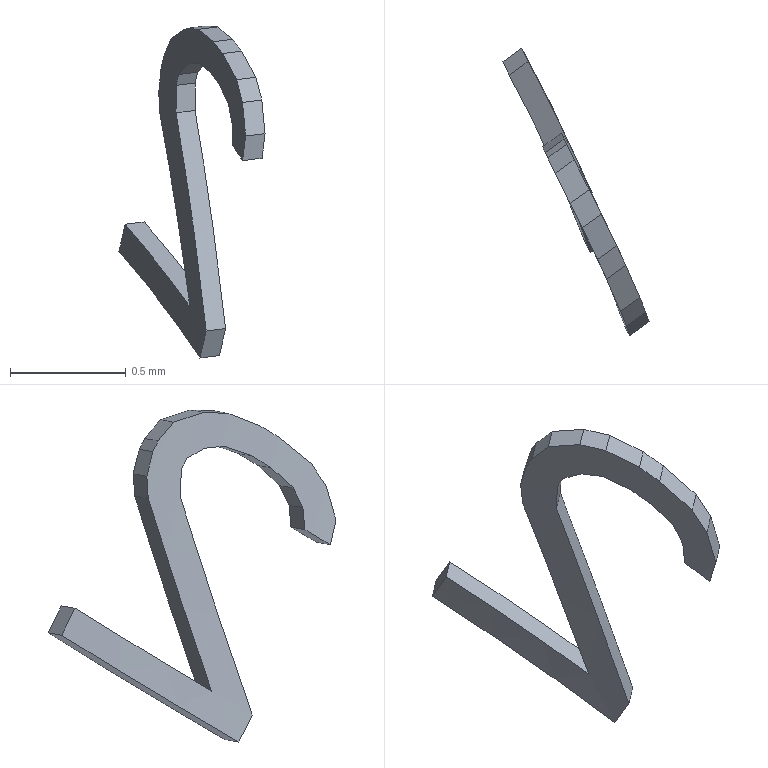Part | SolidWorks | features BaseBody 1 | 1 solid | 30 faces | box 0.631 x 1.244 x 1.435 mm | volume 0.04371 mm3 | plane 28 | cylinder 2 | commonest cylinder face diameters 16.8 x1 17 x1
STEP:
#1=CARTESIAN_POINT('',(1974.074,-240.013,991.84));
#2=VERTEX_POINT('',#1);
#3=CARTESIAN_POINT('',(1973.944,-239.701,992.783));
#4=VERTEX_POINT('',#3);
#5=CARTESIAN_POINT('',(1974.074,-240.013,991.84));
#6=CARTESIAN_POINT('',(1974.04,-239.903,992.154));
#7=CARTESIAN_POINT('',(1973.996,-239.799,992.469));
#8=CARTESIAN_POINT('',(1973.944,-239.701,992.783));
#9=B_SPLINE_CURVE_WITH_KNOTS('',3,(#5,#6,#7,#8),.UNSPECIFIED.,.F.,.F.,(4,4),(0.,1.),.UNSPECIFIED.);
#10=EDGE_CURVE('',#2,#4,#9,.T.);
#11=ORIENTED_EDGE('',*,*,#10,.T.);
#12=CARTESIAN_POINT('',(1973.944,-239.706,992.902));
#13=VERTEX_POINT('',#12);
#14=CARTESIAN_POINT('',(1973.944,-239.701,992.783));
#15=CARTESIAN_POINT('',(1973.944,-239.703,992.823));
#16=CARTESIAN_POINT('',(1973.944,-239.705,992.863));
#17=CARTESIAN_POINT('',(1973.944,-239.706,992.902));
#18=B_SPLINE_CURVE_WITH_KNOTS('',3,(#14,#15,#16,#17),.UNSPECIFIED.,.F.,.F.,(4,4),(0.,1.),.UNSPECIFIED.);
#19=EDGE_CURVE('',#4,#13,#18,.T.);
#20=ORIENTED_EDGE('',*,*,#19,.T.);
#21=CARTESIAN_POINT('',(1973.955,-239.729,992.949));
#22=VERTEX_POINT('',#21);
#23=CARTESIAN_POINT('',(1974.965,-241.915,997.345));
#24=DIRECTION('',(0.2015,-0.436,0.8771));
#25=VECTOR('',#24,1000.);
#26=LINE('',#23,#25);
#27=EDGE_CURVE('',#13,#22,#26,.T.);
#28=ORIENTED_EDGE('',*,*,#27,.T.);
#29=CARTESIAN_POINT('',(1973.992,-239.806,992.993));
#30=VERTEX_POINT('',#29);
#31=CARTESIAN_POINT('',(1973.992,-239.806,992.993));
#32=CARTESIAN_POINT('',(1973.98,-239.78,992.979));
#33=CARTESIAN_POINT('',(1973.967,-239.755,992.964));
#34=CARTESIAN_POINT('',(1973.955,-239.729,992.949));
#35=B_SPLINE_CURVE_WITH_KNOTS('',3,(#31,#32,#33,#34),.UNSPECIFIED.,.F.,.F.,(4,4),(0.,1.),.UNSPECIFIED.);
#36=EDGE_CURVE('',#30,#22,#35,.T.);
#37=ORIENTED_EDGE('',*,*,#36,.F.);
#38=CARTESIAN_POINT('',(1974.033,-239.891,993.002));
#39=VERTEX_POINT('',#38);
#40=CARTESIAN_POINT('',(1974.033,-239.891,993.002));
#41=CARTESIAN_POINT('',(1974.02,-239.863,992.999));
#42=CARTESIAN_POINT('',(1974.006,-239.834,992.996));
#43=CARTESIAN_POINT('',(1973.992,-239.806,992.993));
#44=B_SPLINE_CURVE_WITH_KNOTS('',3,(#40,#41,#42,#43),.UNSPECIFIED.,.F.,.F.,(4,4),(0.,1.),.UNSPECIFIED.);
#45=EDGE_CURVE('',#39,#30,#44,.T.);
#46=ORIENTED_EDGE('',*,*,#45,.F.);
#47=CARTESIAN_POINT('',(1974.089,-240.008,992.961));
#48=VERTEX_POINT('',#47);
#49=CARTESIAN_POINT('',(1974.089,-240.008,992.961));
#50=CARTESIAN_POINT('',(1974.071,-239.969,992.975));
#51=CARTESIAN_POINT('',(1974.052,-239.93,992.988));
#52=CARTESIAN_POINT('',(1974.033,-239.891,993.002));
#53=B_SPLINE_CURVE_WITH_KNOTS('',3,(#49,#50,#51,#52),.UNSPECIFIED.,.F.,.F.,(4,4),(0.,1.),.UNSPECIFIED.);
#54=EDGE_CURVE('',#48,#39,#53,.T.);
#55=ORIENTED_EDGE('',*,*,#54,.F.);
#56=CARTESIAN_POINT('',(1974.128,-240.093,992.91));
#57=VERTEX_POINT('',#56);
#58=CARTESIAN_POINT('',(1966.472,-243.55,992.95));
#59=DIRECTION('',(0.2015,-0.436,0.8771));
#60=DIRECTION('',(-0.7309,-0.6631,-0.1618));
#61=AXIS2_PLACEMENT_3D('',#58,#59,#60);
#62=CIRCLE('',#61,8.4);
#63=EDGE_CURVE('',#57,#48,#62,.T.);
#64=ORIENTED_EDGE('',*,*,#63,.F.);
#65=CARTESIAN_POINT('',(1974.17,-240.189,992.822));
#66=VERTEX_POINT('',#65);
#67=CARTESIAN_POINT('',(1974.17,-240.189,992.822));
#68=CARTESIAN_POINT('',(1974.156,-240.157,992.852));
#69=CARTESIAN_POINT('',(1974.142,-240.125,992.881));
#70=CARTESIAN_POINT('',(1974.128,-240.093,992.91));
#71=B_SPLINE_CURVE_WITH_KNOTS('',3,(#67,#68,#69,#70),.UNSPECIFIED.,.F.,.F.,(4,4),(0.,1.),.UNSPECIFIED.);
#72=EDGE_CURVE('',#66,#57,#71,.T.);
#73=ORIENTED_EDGE('',*,*,#72,.F.);
#74=CARTESIAN_POINT('',(1974.186,-240.231,992.737));
#75=VERTEX_POINT('',#74);
#76=CARTESIAN_POINT('',(1974.186,-240.231,992.737));
#77=CARTESIAN_POINT('',(1974.181,-240.217,992.766));
#78=CARTESIAN_POINT('',(1974.175,-240.203,992.794));
#79=CARTESIAN_POINT('',(1974.17,-240.189,992.822));
#80=B_SPLINE_CURVE_WITH_KNOTS('',3,(#76,#77,#78,#79),.UNSPECIFIED.,.F.,.F.,(4,4),(0.,1.),.UNSPECIFIED.);
#81=EDGE_CURVE('',#75,#66,#80,.T.);
#82=ORIENTED_EDGE('',*,*,#81,.F.);
#83=CARTESIAN_POINT('',(1974.188,-240.24,992.641));
#84=VERTEX_POINT('',#83);
#85=CARTESIAN_POINT('',(1974.188,-240.24,992.641));
#86=CARTESIAN_POINT('',(1974.188,-240.237,992.673));
#87=CARTESIAN_POINT('',(1974.187,-240.234,992.705));
#88=CARTESIAN_POINT('',(1974.186,-240.231,992.737));
#89=B_SPLINE_CURVE_WITH_KNOTS('',3,(#85,#86,#87,#88),.UNSPECIFIED.,.F.,.F.,(4,4),(0.,1.),.UNSPECIFIED.);
#90=EDGE_CURVE('',#84,#75,#89,.T.);
#91=ORIENTED_EDGE('',*,*,#90,.F.);
#92=CARTESIAN_POINT('',(1974.232,-240.35,992.577));
#93=VERTEX_POINT('',#92);
#94=CARTESIAN_POINT('',(1966.44,-243.481,992.81));
#95=DIRECTION('',(0.2015,-0.436,0.8771));
#96=DIRECTION('',(-0.7309,-0.6631,-0.1618));
#97=AXIS2_PLACEMENT_3D('',#94,#95,#96);
#98=CIRCLE('',#97,8.4);
#99=EDGE_CURVE('',#93,#84,#98,.T.);
#100=ORIENTED_EDGE('',*,*,#99,.F.);
#101=CARTESIAN_POINT('',(1974.244,-240.374,992.683));
#102=VERTEX_POINT('',#101);
#103=CARTESIAN_POINT('',(1974.232,-240.35,992.577));
#104=CARTESIAN_POINT('',(1974.236,-240.358,992.612));
#105=CARTESIAN_POINT('',(1974.24,-240.366,992.647));
#106=CARTESIAN_POINT('',(1974.244,-240.374,992.683));
#107=B_SPLINE_CURVE_WITH_KNOTS('',3,(#103,#104,#105,#106),.UNSPECIFIED.,.F.,.F.,(4,4),(0.,1.),.UNSPECIFIED.);
#108=EDGE_CURVE('',#93,#102,#107,.T.);
#109=ORIENTED_EDGE('',*,*,#108,.T.);
#110=CARTESIAN_POINT('',(1974.231,-240.333,992.828));
#111=VERTEX_POINT('',#110);
#112=CARTESIAN_POINT('',(1974.244,-240.374,992.683));
#113=CARTESIAN_POINT('',(1974.24,-240.36,992.731));
#114=CARTESIAN_POINT('',(1974.236,-240.347,992.78));
#115=CARTESIAN_POINT('',(1974.231,-240.333,992.828));
#116=B_SPLINE_CURVE_WITH_KNOTS('',3,(#112,#113,#114,#115),.UNSPECIFIED.,.F.,.F.,(4,4),(0.,1.),.UNSPECIFIED.);
#117=EDGE_CURVE('',#102,#111,#116,.T.);
#118=ORIENTED_EDGE('',*,*,#117,.T.);
#119=CARTESIAN_POINT('',(1974.206,-240.269,992.926));
#120=VERTEX_POINT('',#119);
#121=CARTESIAN_POINT('',(1974.231,-240.333,992.828));
#122=CARTESIAN_POINT('',(1974.223,-240.311,992.861));
#123=CARTESIAN_POINT('',(1974.214,-240.29,992.893));
#124=CARTESIAN_POINT('',(1974.206,-240.269,992.926));
#125=B_SPLINE_CURVE_WITH_KNOTS('',3,(#121,#122,#123,#124),.UNSPECIFIED.,.F.,.F.,(4,4),(0.,1.),.UNSPECIFIED.);
#126=EDGE_CURVE('',#111,#120,#125,.T.);
#127=ORIENTED_EDGE('',*,*,#126,.T.);
#128=CARTESIAN_POINT('',(1974.145,-240.13,993.039));
#129=VERTEX_POINT('',#128);
#130=CARTESIAN_POINT('',(1974.206,-240.269,992.926));
#131=CARTESIAN_POINT('',(1974.186,-240.222,992.964));
#132=CARTESIAN_POINT('',(1974.166,-240.176,993.002));
#133=CARTESIAN_POINT('',(1974.145,-240.13,993.039));
#134=B_SPLINE_CURVE_WITH_KNOTS('',3,(#130,#131,#132,#133),.UNSPECIFIED.,.F.,.F.,(4,4),(0.,1.),.UNSPECIFIED.);
#135=EDGE_CURVE('',#120,#129,#134,.T.);
#136=ORIENTED_EDGE('',*,*,#135,.T.);
#137=CARTESIAN_POINT('',(1974.106,-240.045,993.091));
#138=VERTEX_POINT('',#137);
#139=CARTESIAN_POINT('',(1966.499,-243.608,993.067));
#140=DIRECTION('',(0.2015,-0.436,0.8771));
#141=DIRECTION('',(-0.7309,-0.6631,-0.1618));
#142=AXIS2_PLACEMENT_3D('',#139,#140,#141);
#143=CIRCLE('',#142,8.4);
#144=EDGE_CURVE('',#129,#138,#143,.T.);
#145=ORIENTED_EDGE('',*,*,#144,.T.);
#146=CARTESIAN_POINT('',(1974.04,-239.908,993.144));
#147=VERTEX_POINT('',#146);
#148=CARTESIAN_POINT('',(1974.106,-240.045,993.091));
#149=CARTESIAN_POINT('',(1974.084,-239.999,993.108));
#150=CARTESIAN_POINT('',(1974.062,-239.953,993.126));
#151=CARTESIAN_POINT('',(1974.04,-239.908,993.144));
#152=B_SPLINE_CURVE_WITH_KNOTS('',3,(#148,#149,#150,#151),.UNSPECIFIED.,.F.,.F.,(4,4),(0.,1.),.UNSPECIFIED.);
#153=EDGE_CURVE('',#138,#147,#152,.T.);
#154=ORIENTED_EDGE('',*,*,#153,.T.);
#155=CARTESIAN_POINT('',(1973.987,-239.802,993.148));
#156=VERTEX_POINT('',#155);
#157=CARTESIAN_POINT('',(1974.04,-239.908,993.144));
#158=CARTESIAN_POINT('',(1974.022,-239.872,993.145));
#159=CARTESIAN_POINT('',(1974.005,-239.837,993.147));
#160=CARTESIAN_POINT('',(1973.987,-239.802,993.148));
#161=B_SPLINE_CURVE_WITH_KNOTS('',3,(#157,#158,#159,#160),.UNSPECIFIED.,.F.,.F.,(4,4),(0.,1.),.UNSPECIFIED.);
#162=EDGE_CURVE('',#147,#156,#161,.T.);
#163=ORIENTED_EDGE('',*,*,#162,.T.);
#164=CARTESIAN_POINT('',(1973.923,-239.673,993.106));
#165=VERTEX_POINT('',#164);
#166=CARTESIAN_POINT('',(1973.987,-239.802,993.148));
#167=CARTESIAN_POINT('',(1973.966,-239.759,993.134));
#168=CARTESIAN_POINT('',(1973.944,-239.716,993.12));
#169=CARTESIAN_POINT('',(1973.923,-239.673,993.106));
#170=B_SPLINE_CURVE_WITH_KNOTS('',3,(#166,#167,#168,#169),.UNSPECIFIED.,.F.,.F.,(4,4),(0.,1.),.UNSPECIFIED.);
#171=EDGE_CURVE('',#156,#165,#170,.T.);
#172=ORIENTED_EDGE('',*,*,#171,.T.);
#173=CARTESIAN_POINT('',(1973.89,-239.606,993.025));
#174=VERTEX_POINT('',#173);
#175=CARTESIAN_POINT('',(1973.923,-239.673,993.106));
#176=CARTESIAN_POINT('',(1973.912,-239.651,993.079));
#177=CARTESIAN_POINT('',(1973.901,-239.628,993.052));
#178=CARTESIAN_POINT('',(1973.89,-239.606,993.025));
#179=B_SPLINE_CURVE_WITH_KNOTS('',3,(#175,#176,#177,#178),.UNSPECIFIED.,.F.,.F.,(4,4),(0.,1.),.UNSPECIFIED.);
#180=EDGE_CURVE('',#165,#174,#179,.T.);
#181=ORIENTED_EDGE('',*,*,#180,.T.);
#182=CARTESIAN_POINT('',(1973.879,-239.583,992.978));
#183=VERTEX_POINT('',#182);
#184=CARTESIAN_POINT('',(1974.9,-241.792,997.421));
#185=DIRECTION('',(-0.2015,0.436,-0.8771));
#186=VECTOR('',#185,1000.);
#187=LINE('',#184,#186);
#188=EDGE_CURVE('',#174,#183,#187,.T.);
#189=ORIENTED_EDGE('',*,*,#188,.T.);
#190=CARTESIAN_POINT('',(1973.869,-239.557,992.872));
#191=VERTEX_POINT('',#190);
#192=CARTESIAN_POINT('',(1973.869,-239.557,992.872));
#193=CARTESIAN_POINT('',(1973.872,-239.566,992.908));
#194=CARTESIAN_POINT('',(1973.876,-239.574,992.943));
#195=CARTESIAN_POINT('',(1973.879,-239.583,992.978));
#196=B_SPLINE_CURVE_WITH_KNOTS('',3,(#192,#193,#194,#195),.UNSPECIFIED.,.F.,.F.,(4,4),(0.,1.),.UNSPECIFIED.);
#197=EDGE_CURVE('',#191,#183,#196,.T.);
#198=ORIENTED_EDGE('',*,*,#197,.F.);
#199=CARTESIAN_POINT('',(1973.875,-239.563,992.777));
#200=VERTEX_POINT('',#199);
#201=CARTESIAN_POINT('',(1973.875,-239.563,992.777));
#202=CARTESIAN_POINT('',(1973.873,-239.561,992.809));
#203=CARTESIAN_POINT('',(1973.871,-239.559,992.84));
#204=CARTESIAN_POINT('',(1973.869,-239.557,992.872));
#205=B_SPLINE_CURVE_WITH_KNOTS('',3,(#201,#202,#203,#204),.UNSPECIFIED.,.F.,.F.,(4,4),(0.,1.),.UNSPECIFIED.);
#206=EDGE_CURVE('',#200,#191,#205,.T.);
#207=ORIENTED_EDGE('',*,*,#206,.F.);
#208=CARTESIAN_POINT('',(1974.004,-239.837,991.944));
#209=VERTEX_POINT('',#208);
#210=CARTESIAN_POINT('',(1974.004,-239.837,991.944));
#211=CARTESIAN_POINT('',(1973.968,-239.741,992.221));
#212=CARTESIAN_POINT('',(1973.925,-239.65,992.499));
#213=CARTESIAN_POINT('',(1973.875,-239.563,992.777));
#214=B_SPLINE_CURVE_WITH_KNOTS('',3,(#210,#211,#212,#213),.UNSPECIFIED.,.F.,.F.,(4,4),(0.,1.),.UNSPECIFIED.);
#215=EDGE_CURVE('',#209,#200,#214,.T.);
#216=ORIENTED_EDGE('',*,*,#215,.F.);
#217=CARTESIAN_POINT('',(1973.724,-239.247,992.302));
#218=VERTEX_POINT('',#217);
#219=CARTESIAN_POINT('',(1966.274,-243.121,992.087));
#220=DIRECTION('',(0.2015,-0.436,0.8771));
#221=DIRECTION('',(-0.7309,-0.6631,-0.1618));
#222=AXIS2_PLACEMENT_3D('',#219,#220,#221);
#223=CIRCLE('',#222,8.4);
#224=EDGE_CURVE('',#209,#218,#223,.T.);
#225=ORIENTED_EDGE('',*,*,#224,.T.);
#226=CARTESIAN_POINT('',(1973.697,-239.189,992.185));
#227=VERTEX_POINT('',#226);
#228=CARTESIAN_POINT('',(1974.9,-241.792,997.421));
#229=DIRECTION('',(-0.2015,0.436,-0.8771));
#230=VECTOR('',#229,1000.);
#231=LINE('',#228,#230);
#232=EDGE_CURVE('',#218,#227,#231,.T.);
#233=ORIENTED_EDGE('',*,*,#232,.T.);
#234=CARTESIAN_POINT('',(1974.047,-239.955,991.724));
#235=VERTEX_POINT('',#234);
#236=CARTESIAN_POINT('',(1966.247,-243.063,991.97));
#237=DIRECTION('',(-0.2015,0.436,-0.8771));
#238=DIRECTION('',(-0.7309,-0.6631,-0.1618));
#239=AXIS2_PLACEMENT_3D('',#236,#237,#238);
#240=CIRCLE('',#239,8.4);
#241=EDGE_CURVE('',#227,#235,#240,.T.);
#242=ORIENTED_EDGE('',*,*,#241,.T.);
#243=CARTESIAN_POINT('',(1975.25,-242.558,996.96));
#244=DIRECTION('',(0.2015,-0.436,0.8771));
#245=VECTOR('',#244,1000.);
#246=LINE('',#243,#245);
#247=EDGE_CURVE('',#235,#2,#246,.T.);
#248=ORIENTED_EDGE('',*,*,#247,.T.);
#249=EDGE_LOOP('',(#11,#20,#28,#37,#46,#55,#64,#73,#82,#91,#100,#109,#118,#127,#136,#145,#154,#163,#172,#181,#189,#198,#207,#216,#225,#233,#242,#248));
#250=FACE_OUTER_BOUND('',#249,.T.);
#251=CARTESIAN_POINT('',(1967.45,-245.666,997.207));
#252=DIRECTION('',(0.2015,-0.436,0.8771));
#253=DIRECTION('',(-0.7309,-0.6631,-0.1618));
#254=AXIS2_PLACEMENT_3D('',#251,#252,#253);
#255=CYLINDRICAL_SURFACE('',#254,8.4);
#256=ADVANCED_FACE('',(#250),#255,.F.);
#257=CARTESIAN_POINT('',(1974.158,-239.953,991.851));
#258=VERTEX_POINT('',#257);
#259=CARTESIAN_POINT('',(1974.116,-239.983,991.846));
#260=DIRECTION('',(-0.8088,-0.5792,-0.1022));
#261=VECTOR('',#260,1000.);
#262=LINE('',#259,#261);
#263=EDGE_CURVE('',#258,#2,#262,.T.);
#264=ORIENTED_EDGE('',*,*,#263,.T.);
#265=ORIENTED_EDGE('',*,*,#247,.F.);
#266=CARTESIAN_POINT('',(1974.131,-239.895,991.734));
#267=VERTEX_POINT('',#266);
#268=CARTESIAN_POINT('',(1974.089,-239.925,991.729));
#269=DIRECTION('',(-0.8088,-0.5792,-0.1022));
#270=VECTOR('',#269,1000.);
#271=LINE('',#268,#270);
#272=EDGE_CURVE('',#267,#235,#271,.T.);
#273=ORIENTED_EDGE('',*,*,#272,.F.);
#274=CARTESIAN_POINT('',(1974.145,-239.924,991.793));
#275=DIRECTION('',(0.2015,-0.436,0.8771));
#276=VECTOR('',#275,1000.);
#277=LINE('',#274,#276);
#278=EDGE_CURVE('',#267,#258,#277,.T.);
#279=ORIENTED_EDGE('',*,*,#278,.T.);
#280=EDGE_LOOP('',(#264,#265,#273,#279));
#281=FACE_OUTER_BOUND('',#280,.T.);
#282=CARTESIAN_POINT('',(1979.641,-235.949,992.431));
#283=DIRECTION('',(0.5526,-0.6888,-0.4693));
#284=DIRECTION('',(-0.2015,0.436,-0.8771));
#285=AXIS2_PLACEMENT_3D('',#282,#283,#284);
#286=PLANE('',#285);
#287=ADVANCED_FACE('',(#281),#286,.T.);
#288=ORIENTED_EDGE('',*,*,#272,.T.);
#289=ORIENTED_EDGE('',*,*,#241,.F.);
#290=CARTESIAN_POINT('',(1973.779,-239.13,992.195));
#291=VERTEX_POINT('',#290);
#292=CARTESIAN_POINT('',(1973.738,-239.159,992.19));
#293=DIRECTION('',(-0.8088,-0.5792,-0.1022));
#294=VECTOR('',#293,1000.);
#295=LINE('',#292,#294);
#296=EDGE_CURVE('',#291,#227,#295,.T.);
#297=ORIENTED_EDGE('',*,*,#296,.F.);
#298=CARTESIAN_POINT('',(1966.247,-243.063,991.97));
#299=DIRECTION('',(-0.2015,0.436,-0.8771));
#300=DIRECTION('',(-0.7309,-0.6631,-0.1618));
#301=AXIS2_PLACEMENT_3D('',#298,#299,#300);
#302=CIRCLE('',#301,8.5);
#303=EDGE_CURVE('',#291,#267,#302,.T.);
#304=ORIENTED_EDGE('',*,*,#303,.T.);
#305=EDGE_LOOP('',(#288,#289,#297,#304));
#306=FACE_OUTER_BOUND('',#305,.T.);
#307=CARTESIAN_POINT('',(1981.656,-238.46,990.719));
#308=DIRECTION('',(-0.2015,0.436,-0.8771));
#309=DIRECTION('',(-0.5526,0.6888,0.4693));
#310=AXIS2_PLACEMENT_3D('',#307,#308,#309);
#311=PLANE('',#310);
#312=ADVANCED_FACE('',(#306),#311,.T.);
#313=ORIENTED_EDGE('',*,*,#296,.T.);
#314=ORIENTED_EDGE('',*,*,#232,.F.);
#315=CARTESIAN_POINT('',(1973.806,-239.188,992.312));
#316=VERTEX_POINT('',#315);
#317=CARTESIAN_POINT('',(1973.765,-239.217,992.307));
#318=DIRECTION('',(-0.8088,-0.5792,-0.1022));
#319=VECTOR('',#318,1000.);
#320=LINE('',#317,#319);
#321=EDGE_CURVE('',#316,#218,#320,.T.);
#322=ORIENTED_EDGE('',*,*,#321,.F.);
#323=CARTESIAN_POINT('',(1973.793,-239.159,992.254));
#324=DIRECTION('',(-0.2015,0.436,-0.8771));
#325=VECTOR('',#324,1000.);
#326=LINE('',#323,#325);
#327=EDGE_CURVE('',#316,#291,#326,.T.);
#328=ORIENTED_EDGE('',*,*,#327,.T.);
#329=EDGE_LOOP('',(#313,#314,#322,#328));
#330=FACE_OUTER_BOUND('',#329,.T.);
#331=CARTESIAN_POINT('',(1979.15,-235.361,992.987));
#332=DIRECTION('',(-0.5526,0.6888,0.4693));
#333=DIRECTION('',(0.2015,-0.436,0.8771));
#334=AXIS2_PLACEMENT_3D('',#331,#332,#333);
#335=PLANE('',#334);
#336=ADVANCED_FACE('',(#330),#335,.T.);
#337=ORIENTED_EDGE('',*,*,#321,.T.);
#338=ORIENTED_EDGE('',*,*,#224,.F.);
#339=CARTESIAN_POINT('',(1974.088,-239.777,991.955));
#340=VERTEX_POINT('',#339);
#341=CARTESIAN_POINT('',(1974.046,-239.807,991.949));
#342=DIRECTION('',(-0.8088,-0.5792,-0.1022));
#343=VECTOR('',#342,1000.);
#344=LINE('',#341,#343);
#345=EDGE_CURVE('',#340,#209,#344,.T.);
#346=ORIENTED_EDGE('',*,*,#345,.F.);
#347=CARTESIAN_POINT('',(1966.274,-243.121,992.087));
#348=DIRECTION('',(0.2015,-0.436,0.8771));
#349=DIRECTION('',(-0.7309,-0.6631,-0.1618));
#350=AXIS2_PLACEMENT_3D('',#347,#348,#349);
#351=CIRCLE('',#350,8.5);
#352=EDGE_CURVE('',#340,#316,#351,.T.);
#353=ORIENTED_EDGE('',*,*,#352,.T.);
#354=EDGE_LOOP('',(#337,#338,#346,#353));
#355=FACE_OUTER_BOUND('',#354,.T.);
#356=CARTESIAN_POINT('',(1976.862,-232.509,994.931));
#357=DIRECTION('',(0.2015,-0.436,0.8771));
#358=DIRECTION('',(0.5526,-0.6888,-0.4693));
#359=AXIS2_PLACEMENT_3D('',#356,#357,#358);
#360=PLANE('',#359);
#361=ADVANCED_FACE('',(#355),#360,.T.);
#362=ORIENTED_EDGE('',*,*,#345,.T.);
#363=ORIENTED_EDGE('',*,*,#215,.T.);
#364=CARTESIAN_POINT('',(1973.957,-239.504,992.787));
#365=VERTEX_POINT('',#364);
#366=CARTESIAN_POINT('',(1973.916,-239.534,992.782));
#367=DIRECTION('',(-0.8088,-0.5792,-0.1022));
#368=VECTOR('',#367,1000.);
#369=LINE('',#366,#368);
#370=EDGE_CURVE('',#365,#200,#369,.T.);
#371=ORIENTED_EDGE('',*,*,#370,.F.);
#372=CARTESIAN_POINT('',(1974.088,-239.777,991.955));
#373=CARTESIAN_POINT('',(1974.066,-239.72,992.121));
#374=CARTESIAN_POINT('',(1974.042,-239.664,992.287));
#375=CARTESIAN_POINT('',(1974.016,-239.609,992.454));
#376=CARTESIAN_POINT('',(1973.987,-239.556,992.621));
#377=CARTESIAN_POINT('',(1973.957,-239.504,992.787));
#378=B_SPLINE_CURVE_WITH_KNOTS('',5,(#372,#373,#374,#375,#376,#377),.UNSPECIFIED.,.F.,.F.,(6,6),(0.,1.),.UNSPECIFIED.);
#379=EDGE_CURVE('',#340,#365,#378,.T.);
#380=ORIENTED_EDGE('',*,*,#379,.F.);
#381=EDGE_LOOP('',(#362,#363,#371,#380));
#382=FACE_OUTER_BOUND('',#381,.T.);
#383=CARTESIAN_POINT('',(1979.311,-235.67,993.464));
#384=DIRECTION('',(-0.5192,0.7847,-0.3386));
#385=DIRECTION('',(-0.2763,0.2208,0.9354));
#386=AXIS2_PLACEMENT_3D('',#383,#384,#385);
#387=PLANE('',#386);
#388=ADVANCED_FACE('',(#382),#387,.T.);
#389=ORIENTED_EDGE('',*,*,#370,.T.);
#390=ORIENTED_EDGE('',*,*,#206,.T.);
#391=CARTESIAN_POINT('',(1973.951,-239.498,992.883));
#392=VERTEX_POINT('',#391);
#393=CARTESIAN_POINT('',(1973.91,-239.528,992.877));
#394=DIRECTION('',(-0.8088,-0.5792,-0.1022));
#395=VECTOR('',#394,1000.);
#396=LINE('',#393,#395);
#397=EDGE_CURVE('',#392,#191,#396,.T.);
#398=ORIENTED_EDGE('',*,*,#397,.F.);
#399=CARTESIAN_POINT('',(1973.957,-239.504,992.787));
#400=CARTESIAN_POINT('',(1973.956,-239.503,992.806));
#401=CARTESIAN_POINT('',(1973.954,-239.502,992.825));
#402=CARTESIAN_POINT('',(1973.953,-239.501,992.844));
#403=CARTESIAN_POINT('',(1973.952,-239.5,992.864));
#404=CARTESIAN_POINT('',(1973.951,-239.498,992.883));
#405=B_SPLINE_CURVE_WITH_KNOTS('',5,(#399,#400,#401,#402,#403,#404),.UNSPECIFIED.,.F.,.F.,(6,6),(0.,1.),.UNSPECIFIED.);
#406=EDGE_CURVE('',#365,#392,#405,.T.);
#407=ORIENTED_EDGE('',*,*,#406,.F.);
#408=EDGE_LOOP('',(#389,#390,#398,#407));
#409=FACE_OUTER_BOUND('',#408,.T.);
#410=CARTESIAN_POINT('',(1979.298,-235.669,993.558));
#411=DIRECTION('',(-0.5728,0.8151,-0.08642));
#412=DIRECTION('',(-0.1333,0.01137,0.991));
#413=AXIS2_PLACEMENT_3D('',#410,#411,#412);
#414=PLANE('',#413);
#415=ADVANCED_FACE('',(#409),#414,.T.);
#416=ORIENTED_EDGE('',*,*,#397,.T.);
#417=ORIENTED_EDGE('',*,*,#197,.T.);
#418=CARTESIAN_POINT('',(1973.961,-239.524,992.989));
#419=VERTEX_POINT('',#418);
#420=CARTESIAN_POINT('',(1973.92,-239.554,992.983));
#421=DIRECTION('',(-0.8088,-0.5792,-0.1022));
#422=VECTOR('',#421,1000.);
#423=LINE('',#420,#422);
#424=EDGE_CURVE('',#419,#183,#423,.T.);
#425=ORIENTED_EDGE('',*,*,#424,.F.);
#426=CARTESIAN_POINT('',(1973.951,-239.498,992.883));
#427=CARTESIAN_POINT('',(1973.953,-239.504,992.904));
#428=CARTESIAN_POINT('',(1973.955,-239.509,992.925));
#429=CARTESIAN_POINT('',(1973.957,-239.514,992.946));
#430=CARTESIAN_POINT('',(1973.959,-239.519,992.967));
#431=CARTESIAN_POINT('',(1973.961,-239.524,992.989));
#432=B_SPLINE_CURVE_WITH_KNOTS('',5,(#426,#427,#428,#429,#430,#431),.UNSPECIFIED.,.F.,.F.,(6,6),(0.,1.),.UNSPECIFIED.);
#433=EDGE_CURVE('',#392,#419,#432,.T.);
#434=ORIENTED_EDGE('',*,*,#433,.F.);
#435=EDGE_LOOP('',(#416,#417,#425,#434));
#436=FACE_OUTER_BOUND('',#435,.T.);
#437=CARTESIAN_POINT('',(1979.305,-235.697,993.664));
#438=DIRECTION('',(-0.5846,0.7727,0.2473));
#439=DIRECTION('',(0.06431,-0.2598,0.9635));
#440=AXIS2_PLACEMENT_3D('',#437,#438,#439);
#441=PLANE('',#440);
#442=ADVANCED_FACE('',(#436),#441,.T.);
#443=ORIENTED_EDGE('',*,*,#424,.T.);
#444=ORIENTED_EDGE('',*,*,#188,.F.);
#445=CARTESIAN_POINT('',(1973.972,-239.548,993.035));
#446=VERTEX_POINT('',#445);
#447=CARTESIAN_POINT('',(1973.931,-239.577,993.03));
#448=DIRECTION('',(-0.8088,-0.5792,-0.1022));
#449=VECTOR('',#448,1000.);
#450=LINE('',#447,#449);
#451=EDGE_CURVE('',#446,#174,#450,.T.);
#452=ORIENTED_EDGE('',*,*,#451,.F.);
#453=CARTESIAN_POINT('',(1973.967,-239.536,993.012));
#454=DIRECTION('',(-0.2015,0.436,-0.8771));
#455=VECTOR('',#454,1000.);
#456=LINE('',#453,#455);
#457=EDGE_CURVE('',#446,#419,#456,.T.);
#458=ORIENTED_EDGE('',*,*,#457,.T.);
#459=EDGE_LOOP('',(#443,#444,#452,#458));
#460=FACE_OUTER_BOUND('',#459,.T.);
#461=CARTESIAN_POINT('',(1979.15,-235.361,992.987));
#462=DIRECTION('',(-0.5526,0.6888,0.4693));
#463=DIRECTION('',(0.2015,-0.436,0.8771));
#464=AXIS2_PLACEMENT_3D('',#461,#462,#463);
#465=PLANE('',#464);
#466=ADVANCED_FACE('',(#460),#465,.T.);
#467=ORIENTED_EDGE('',*,*,#451,.T.);
#468=ORIENTED_EDGE('',*,*,#180,.F.);
#469=CARTESIAN_POINT('',(1974.005,-239.614,993.116));
#470=VERTEX_POINT('',#469);
#471=CARTESIAN_POINT('',(1973.964,-239.644,993.111));
#472=DIRECTION('',(-0.8088,-0.5792,-0.1022));
#473=VECTOR('',#472,1000.);
#474=LINE('',#471,#473);
#475=EDGE_CURVE('',#470,#165,#474,.T.);
#476=ORIENTED_EDGE('',*,*,#475,.F.);
#477=CARTESIAN_POINT('',(1974.005,-239.614,993.116));
#478=CARTESIAN_POINT('',(1973.998,-239.601,993.1));
#479=CARTESIAN_POINT('',(1973.992,-239.588,993.084));
#480=CARTESIAN_POINT('',(1973.985,-239.574,993.067));
#481=CARTESIAN_POINT('',(1973.979,-239.561,993.051));
#482=CARTESIAN_POINT('',(1973.972,-239.548,993.035));
#483=B_SPLINE_CURVE_WITH_KNOTS('',5,(#477,#478,#479,#480,#481,#482),.UNSPECIFIED.,.F.,.F.,(6,6),(0.,1.),.UNSPECIFIED.);
#484=EDGE_CURVE('',#470,#446,#483,.T.);
#485=ORIENTED_EDGE('',*,*,#484,.T.);
#486=EDGE_LOOP('',(#467,#468,#476,#485));
#487=FACE_OUTER_BOUND('',#486,.T.);
#488=CARTESIAN_POINT('',(1979.352,-235.785,993.791));
#489=DIRECTION('',(-0.4888,0.5653,0.6644));
#490=DIRECTION('',(0.3271,-0.5873,0.7403));
#491=AXIS2_PLACEMENT_3D('',#488,#489,#490);
#492=PLANE('',#491);
#493=ADVANCED_FACE('',(#487),#492,.T.);
#494=ORIENTED_EDGE('',*,*,#475,.T.);
#495=ORIENTED_EDGE('',*,*,#171,.F.);
#496=CARTESIAN_POINT('',(1974.069,-239.743,993.158));
#497=VERTEX_POINT('',#496);
#498=CARTESIAN_POINT('',(1974.028,-239.772,993.153));
#499=DIRECTION('',(-0.8088,-0.5792,-0.1022));
#500=VECTOR('',#499,1000.);
#501=LINE('',#498,#500);
#502=EDGE_CURVE('',#497,#156,#501,.T.);
#503=ORIENTED_EDGE('',*,*,#502,.F.);
#504=CARTESIAN_POINT('',(1974.069,-239.743,993.158));
#505=CARTESIAN_POINT('',(1974.056,-239.717,993.15));
#506=CARTESIAN_POINT('',(1974.043,-239.691,993.141));
#507=CARTESIAN_POINT('',(1974.031,-239.666,993.133));
#508=CARTESIAN_POINT('',(1974.018,-239.64,993.124));
#509=CARTESIAN_POINT('',(1974.005,-239.614,993.116));
#510=B_SPLINE_CURVE_WITH_KNOTS('',5,(#504,#505,#506,#507,#508,#509),.UNSPECIFIED.,.F.,.F.,(6,6),(0.,1.),.UNSPECIFIED.);
#511=EDGE_CURVE('',#497,#470,#510,.T.);
#512=ORIENTED_EDGE('',*,*,#511,.T.);
#513=EDGE_LOOP('',(#494,#495,#503,#512));
#514=FACE_OUTER_BOUND('',#513,.T.);
#515=CARTESIAN_POINT('',(1979.431,-235.903,993.836));
#516=DIRECTION('',(-0.2539,0.1871,0.949));
#517=DIRECTION('',(0.5305,-0.7934,0.2983));
#518=AXIS2_PLACEMENT_3D('',#515,#516,#517);
#519=PLANE('',#518);
#520=ADVANCED_FACE('',(#514),#519,.T.);
#521=ORIENTED_EDGE('',*,*,#502,.T.);
#522=ORIENTED_EDGE('',*,*,#162,.F.);
#523=CARTESIAN_POINT('',(1974.122,-239.849,993.154));
#524=VERTEX_POINT('',#523);
#525=CARTESIAN_POINT('',(1974.081,-239.878,993.149));
#526=DIRECTION('',(-0.8088,-0.5792,-0.1022));
#527=VECTOR('',#526,1000.);
#528=LINE('',#525,#527);
#529=EDGE_CURVE('',#524,#147,#528,.T.);
#530=ORIENTED_EDGE('',*,*,#529,.F.);
#531=CARTESIAN_POINT('',(1974.122,-239.849,993.154));
#532=CARTESIAN_POINT('',(1974.112,-239.827,993.155));
#533=CARTESIAN_POINT('',(1974.101,-239.806,993.156));
#534=CARTESIAN_POINT('',(1974.091,-239.785,993.157));
#535=CARTESIAN_POINT('',(1974.08,-239.764,993.158));
#536=CARTESIAN_POINT('',(1974.069,-239.743,993.158));
#537=B_SPLINE_CURVE_WITH_KNOTS('',5,(#531,#532,#533,#534,#535,#536),.UNSPECIFIED.,.F.,.F.,(6,6),(0.,1.),.UNSPECIFIED.);
#538=EDGE_CURVE('',#524,#497,#537,.T.);
#539=ORIENTED_EDGE('',*,*,#538,.T.);
#540=EDGE_LOOP('',(#521,#522,#530,#539));
#541=FACE_OUTER_BOUND('',#540,.T.);
#542=CARTESIAN_POINT('',(1979.499,-235.998,993.834));
#543=DIRECTION('',(-0.07187,-0.07511,0.9946));
#544=DIRECTION('',(0.5837,-0.8117,-0.01912));
#545=AXIS2_PLACEMENT_3D('',#542,#543,#544);
#546=PLANE('',#545);
#547=ADVANCED_FACE('',(#541),#546,.T.);
#548=ORIENTED_EDGE('',*,*,#529,.T.);
#549=ORIENTED_EDGE('',*,*,#153,.F.);
#550=CARTESIAN_POINT('',(1974.189,-239.986,993.101));
#551=VERTEX_POINT('',#550);
#552=CARTESIAN_POINT('',(1974.147,-240.016,993.096));
#553=DIRECTION('',(-0.8088,-0.5792,-0.1022));
#554=VECTOR('',#553,1000.);
#555=LINE('',#552,#554);
#556=EDGE_CURVE('',#551,#138,#555,.T.);
#557=ORIENTED_EDGE('',*,*,#556,.F.);
#558=CARTESIAN_POINT('',(1974.189,-239.986,993.101));
#559=CARTESIAN_POINT('',(1974.176,-239.958,993.112));
#560=CARTESIAN_POINT('',(1974.162,-239.931,993.122));
#561=CARTESIAN_POINT('',(1974.149,-239.903,993.133));
#562=CARTESIAN_POINT('',(1974.136,-239.876,993.144));
#563=CARTESIAN_POINT('',(1974.122,-239.849,993.154));
#564=B_SPLINE_CURVE_WITH_KNOTS('',5,(#558,#559,#560,#561,#562,#563),.UNSPECIFIED.,.F.,.F.,(6,6),(0.,1.),.UNSPECIFIED.);
#565=EDGE_CURVE('',#551,#524,#564,.T.);
#566=ORIENTED_EDGE('',*,*,#565,.T.);
#567=EDGE_LOOP('',(#548,#549,#557,#566));
#568=FACE_OUTER_BOUND('',#567,.T.);
#569=CARTESIAN_POINT('',(1979.591,-236.117,993.784));
#570=DIRECTION('',(0.1059,-0.3143,0.9434));
#571=DIRECTION('',(0.5785,-0.7522,-0.3155));
#572=AXIS2_PLACEMENT_3D('',#569,#570,#571);
#573=PLANE('',#572);
#574=ADVANCED_FACE('',(#568),#573,.T.);
#575=ORIENTED_EDGE('',*,*,#556,.T.);
#576=ORIENTED_EDGE('',*,*,#144,.F.);
#577=CARTESIAN_POINT('',(1974.228,-240.071,993.05));
#578=VERTEX_POINT('',#577);
#579=CARTESIAN_POINT('',(1974.187,-240.1,993.045));
#580=DIRECTION('',(-0.8088,-0.5792,-0.1022));
#581=VECTOR('',#580,1000.);
#582=LINE('',#579,#581);
#583=EDGE_CURVE('',#578,#129,#582,.T.);
#584=ORIENTED_EDGE('',*,*,#583,.F.);
#585=CARTESIAN_POINT('',(1966.499,-243.608,993.067));
#586=DIRECTION('',(0.2015,-0.436,0.8771));
#587=DIRECTION('',(-0.7309,-0.6631,-0.1618));
#588=AXIS2_PLACEMENT_3D('',#585,#586,#587);
#589=CIRCLE('',#588,8.5);
#590=EDGE_CURVE('',#578,#551,#589,.T.);
#591=ORIENTED_EDGE('',*,*,#590,.T.);
#592=EDGE_LOOP('',(#575,#576,#584,#591));
#593=FACE_OUTER_BOUND('',#592,.T.);
#594=CARTESIAN_POINT('',(1982.253,-239.435,991.522));
#595=DIRECTION('',(0.2015,-0.436,0.8771));
#596=DIRECTION('',(0.5526,-0.6888,-0.4693));
#597=AXIS2_PLACEMENT_3D('',#594,#595,#596);
#598=PLANE('',#597);
#599=ADVANCED_FACE('',(#593),#598,.T.);
#600=ORIENTED_EDGE('',*,*,#583,.T.);
#601=ORIENTED_EDGE('',*,*,#135,.F.);
#602=CARTESIAN_POINT('',(1974.289,-240.209,992.937));
#603=VERTEX_POINT('',#602);
#604=CARTESIAN_POINT('',(1974.247,-240.239,992.931));
#605=DIRECTION('',(-0.8088,-0.5792,-0.1022));
#606=VECTOR('',#605,1000.);
#607=LINE('',#604,#606);
#608=EDGE_CURVE('',#603,#120,#607,.T.);
#609=ORIENTED_EDGE('',*,*,#608,.F.);
#610=CARTESIAN_POINT('',(1974.289,-240.209,992.937));
#611=CARTESIAN_POINT('',(1974.277,-240.181,992.959));
#612=CARTESIAN_POINT('',(1974.265,-240.154,992.982));
#613=CARTESIAN_POINT('',(1974.253,-240.126,993.005));
#614=CARTESIAN_POINT('',(1974.241,-240.098,993.027));
#615=CARTESIAN_POINT('',(1974.228,-240.071,993.05));
#616=B_SPLINE_CURVE_WITH_KNOTS('',5,(#610,#611,#612,#613,#614,#615),.UNSPECIFIED.,.F.,.F.,(6,6),(0.,1.),.UNSPECIFIED.);
#617=EDGE_CURVE('',#603,#578,#616,.T.);
#618=ORIENTED_EDGE('',*,*,#617,.T.);
#619=EDGE_LOOP('',(#600,#601,#609,#618));
#620=FACE_OUTER_BOUND('',#619,.T.);
#621=CARTESIAN_POINT('',(1979.744,-236.303,993.626));
#622=DIRECTION('',(0.2791,-0.5309,0.8001));
#623=DIRECTION('',(0.5177,-0.6186,-0.591));
#624=AXIS2_PLACEMENT_3D('',#621,#622,#623);
#625=PLANE('',#624);
#626=ADVANCED_FACE('',(#620),#625,.T.);
#627=ORIENTED_EDGE('',*,*,#608,.T.);
#628=ORIENTED_EDGE('',*,*,#126,.F.);
#629=CARTESIAN_POINT('',(1974.315,-240.273,992.838));
#630=VERTEX_POINT('',#629);
#631=CARTESIAN_POINT('',(1974.273,-240.303,992.833));
#632=DIRECTION('',(-0.8088,-0.5792,-0.1022));
#633=VECTOR('',#632,1000.);
#634=LINE('',#631,#633);
#635=EDGE_CURVE('',#630,#111,#634,.T.);
#636=ORIENTED_EDGE('',*,*,#635,.F.);
#637=CARTESIAN_POINT('',(1974.315,-240.273,992.838));
#638=CARTESIAN_POINT('',(1974.31,-240.26,992.858));
#639=CARTESIAN_POINT('',(1974.304,-240.247,992.878));
#640=CARTESIAN_POINT('',(1974.299,-240.235,992.897));
#641=CARTESIAN_POINT('',(1974.294,-240.222,992.917));
#642=CARTESIAN_POINT('',(1974.289,-240.209,992.937));
#643=B_SPLINE_CURVE_WITH_KNOTS('',5,(#637,#638,#639,#640,#641,#642),.UNSPECIFIED.,.F.,.F.,(6,6),(0.,1.),.UNSPECIFIED.);
#644=EDGE_CURVE('',#630,#603,#643,.T.);
#645=ORIENTED_EDGE('',*,*,#644,.T.);
#646=EDGE_LOOP('',(#627,#628,#636,#645));
#647=FACE_OUTER_BOUND('',#646,.T.);
#648=CARTESIAN_POINT('',(1979.79,-236.351,993.53));
#649=DIRECTION('',(0.4307,-0.7016,0.5677));
#650=DIRECTION('',(0.4005,-0.4151,-0.8169));
#651=AXIS2_PLACEMENT_3D('',#648,#649,#650);
#652=PLANE('',#651);
#653=ADVANCED_FACE('',(#647),#652,.T.);
#654=ORIENTED_EDGE('',*,*,#635,.T.);
#655=ORIENTED_EDGE('',*,*,#117,.F.);
#656=CARTESIAN_POINT('',(1974.328,-240.314,992.693));
#657=VERTEX_POINT('',#656);
#658=CARTESIAN_POINT('',(1974.286,-240.344,992.688));
#659=DIRECTION('',(-0.8088,-0.5792,-0.1022));
#660=VECTOR('',#659,1000.);
#661=LINE('',#658,#660);
#662=EDGE_CURVE('',#657,#102,#661,.T.);
#663=ORIENTED_EDGE('',*,*,#662,.F.);
#664=CARTESIAN_POINT('',(1974.328,-240.314,992.693));
#665=CARTESIAN_POINT('',(1974.326,-240.306,992.722));
#666=CARTESIAN_POINT('',(1974.323,-240.298,992.751));
#667=CARTESIAN_POINT('',(1974.32,-240.289,992.78));
#668=CARTESIAN_POINT('',(1974.317,-240.281,992.809));
#669=CARTESIAN_POINT('',(1974.315,-240.273,992.838));
#670=B_SPLINE_CURVE_WITH_KNOTS('',5,(#664,#665,#666,#667,#668,#669),.UNSPECIFIED.,.F.,.F.,(6,6),(0.,1.),.UNSPECIFIED.);
#671=EDGE_CURVE('',#657,#630,#670,.T.);
#672=ORIENTED_EDGE('',*,*,#671,.T.);
#673=EDGE_LOOP('',(#654,#655,#663,#672));
#674=FACE_OUTER_BOUND('',#673,.T.);
#675=CARTESIAN_POINT('',(1979.827,-236.377,993.388));
#676=DIRECTION('',(0.5358,-0.7972,0.2783));
#677=DIRECTION('',(0.2426,-0.1703,-0.955));
#678=AXIS2_PLACEMENT_3D('',#675,#676,#677);
#679=PLANE('',#678);
#680=ADVANCED_FACE('',(#674),#679,.T.);
#681=ORIENTED_EDGE('',*,*,#662,.T.);
#682=ORIENTED_EDGE('',*,*,#108,.F.);
#683=CARTESIAN_POINT('',(1974.315,-240.29,992.587));
#684=VERTEX_POINT('',#683);
#685=CARTESIAN_POINT('',(1974.274,-240.32,992.582));
#686=DIRECTION('',(-0.8088,-0.5792,-0.1022));
#687=VECTOR('',#686,1000.);
#688=LINE('',#685,#687);
#689=EDGE_CURVE('',#684,#93,#688,.T.);
#690=ORIENTED_EDGE('',*,*,#689,.F.);
#691=CARTESIAN_POINT('',(1974.315,-240.29,992.587));
#692=CARTESIAN_POINT('',(1974.318,-240.295,992.608));
#693=CARTESIAN_POINT('',(1974.321,-240.3,992.63));
#694=CARTESIAN_POINT('',(1974.323,-240.305,992.651));
#695=CARTESIAN_POINT('',(1974.326,-240.31,992.672));
#696=CARTESIAN_POINT('',(1974.328,-240.314,992.693));
#697=B_SPLINE_CURVE_WITH_KNOTS('',5,(#691,#692,#693,#694,#695,#696),.UNSPECIFIED.,.F.,.F.,(6,6),(0.,1.),.UNSPECIFIED.);
#698=EDGE_CURVE('',#684,#657,#697,.T.);
#699=ORIENTED_EDGE('',*,*,#698,.T.);
#700=EDGE_LOOP('',(#681,#682,#690,#699));
#701=FACE_OUTER_BOUND('',#700,.T.);
#702=CARTESIAN_POINT('',(1979.82,-236.348,993.283));
#703=DIRECTION('',(0.5846,-0.7727,-0.2473));
#704=DIRECTION('',(-0.0643,0.2598,-0.9635));
#705=AXIS2_PLACEMENT_3D('',#702,#703,#704);
#706=PLANE('',#705);
#707=ADVANCED_FACE('',(#701),#706,.T.);
#708=CARTESIAN_POINT('',(1974.272,-240.18,992.652));
#709=VERTEX_POINT('',#708);
#710=CARTESIAN_POINT('',(1966.44,-243.481,992.81));
#711=DIRECTION('',(0.2015,-0.436,0.8771));
#712=DIRECTION('',(-0.7309,-0.6631,-0.1618));
#713=AXIS2_PLACEMENT_3D('',#710,#711,#712);
#714=CIRCLE('',#713,8.5);
#715=EDGE_CURVE('',#684,#709,#714,.T.);
#716=ORIENTED_EDGE('',*,*,#715,.F.);
#717=ORIENTED_EDGE('',*,*,#689,.T.);
#718=ORIENTED_EDGE('',*,*,#99,.T.);
#719=CARTESIAN_POINT('',(1974.23,-240.21,992.647));
#720=DIRECTION('',(-0.8088,-0.5792,-0.1022));
#721=VECTOR('',#720,1000.);
#722=LINE('',#719,#721);
#723=EDGE_CURVE('',#709,#84,#722,.T.);
#724=ORIENTED_EDGE('',*,*,#723,.F.);
#725=EDGE_LOOP('',(#716,#717,#718,#724));
#726=FACE_OUTER_BOUND('',#725,.T.);
#727=CARTESIAN_POINT('',(1976.827,-232.617,995.825));
#728=DIRECTION('',(0.2015,-0.436,0.8771));
#729=DIRECTION('',(0.5526,-0.6888,-0.4693));
#730=AXIS2_PLACEMENT_3D('',#727,#728,#729);
#731=PLANE('',#730);
#732=ADVANCED_FACE('',(#726),#731,.F.);
#733=ORIENTED_EDGE('',*,*,#723,.T.);
#734=ORIENTED_EDGE('',*,*,#90,.T.);
#735=CARTESIAN_POINT('',(1974.27,-240.171,992.748));
#736=VERTEX_POINT('',#735);
#737=CARTESIAN_POINT('',(1974.228,-240.201,992.742));
#738=DIRECTION('',(-0.8088,-0.5792,-0.1022));
#739=VECTOR('',#738,1000.);
#740=LINE('',#737,#739);
#741=EDGE_CURVE('',#736,#75,#740,.T.);
#742=ORIENTED_EDGE('',*,*,#741,.F.);
#743=CARTESIAN_POINT('',(1974.272,-240.18,992.652));
#744=CARTESIAN_POINT('',(1974.271,-240.178,992.671));
#745=CARTESIAN_POINT('',(1974.271,-240.177,992.69));
#746=CARTESIAN_POINT('',(1974.271,-240.175,992.709));
#747=CARTESIAN_POINT('',(1974.27,-240.173,992.728));
#748=CARTESIAN_POINT('',(1974.27,-240.171,992.748));
#749=B_SPLINE_CURVE_WITH_KNOTS('',5,(#743,#744,#745,#746,#747,#748),.UNSPECIFIED.,.F.,.F.,(6,6),(0.,1.),.UNSPECIFIED.);
#750=EDGE_CURVE('',#709,#736,#749,.T.);
#751=ORIENTED_EDGE('',*,*,#750,.F.);
#752=EDGE_LOOP('',(#733,#734,#742,#751));
#753=FACE_OUTER_BOUND('',#752,.T.);
#754=CARTESIAN_POINT('',(1979.735,-236.258,993.438));
#755=DIRECTION('',(-0.5728,0.8151,-0.08642));
#756=DIRECTION('',(-0.1333,0.01136,0.991));
#757=AXIS2_PLACEMENT_3D('',#754,#755,#756);
#758=PLANE('',#757);
#759=ADVANCED_FACE('',(#753),#758,.T.);
#760=ORIENTED_EDGE('',*,*,#741,.T.);
#761=ORIENTED_EDGE('',*,*,#81,.T.);
#762=CARTESIAN_POINT('',(1974.253,-240.13,992.833));
#763=VERTEX_POINT('',#762);
#764=CARTESIAN_POINT('',(1974.211,-240.16,992.828));
#765=DIRECTION('',(-0.8088,-0.5792,-0.1022));
#766=VECTOR('',#765,1000.);
#767=LINE('',#764,#766);
#768=EDGE_CURVE('',#763,#66,#767,.T.);
#769=ORIENTED_EDGE('',*,*,#768,.F.);
#770=CARTESIAN_POINT('',(1974.27,-240.171,992.748));
#771=CARTESIAN_POINT('',(1974.266,-240.163,992.765));
#772=CARTESIAN_POINT('',(1974.263,-240.155,992.782));
#773=CARTESIAN_POINT('',(1974.26,-240.146,992.799));
#774=CARTESIAN_POINT('',(1974.256,-240.138,992.816));
#775=CARTESIAN_POINT('',(1974.253,-240.13,992.833));
#776=B_SPLINE_CURVE_WITH_KNOTS('',5,(#770,#771,#772,#773,#774,#775),.UNSPECIFIED.,.F.,.F.,(6,6),(0.,1.),.UNSPECIFIED.);
#777=EDGE_CURVE('',#736,#763,#776,.T.);
#778=ORIENTED_EDGE('',*,*,#777,.F.);
#779=EDGE_LOOP('',(#760,#761,#769,#778));
#780=FACE_OUTER_BOUND('',#779,.T.);
#781=CARTESIAN_POINT('',(1979.702,-236.227,993.521));
#782=DIRECTION('',(-0.4775,0.7481,-0.4609));
#783=DIRECTION('',(-0.3434,0.3239,0.8816));
#784=AXIS2_PLACEMENT_3D('',#781,#782,#783);
#785=PLANE('',#784);
#786=ADVANCED_FACE('',(#780),#785,.T.);
#787=ORIENTED_EDGE('',*,*,#768,.T.);
#788=ORIENTED_EDGE('',*,*,#72,.T.);
#789=CARTESIAN_POINT('',(1974.211,-240.034,992.92));
#790=VERTEX_POINT('',#789);
#791=CARTESIAN_POINT('',(1974.169,-240.064,992.915));
#792=DIRECTION('',(-0.8088,-0.5792,-0.1022));
#793=VECTOR('',#792,1000.);
#794=LINE('',#791,#793);
#795=EDGE_CURVE('',#790,#57,#794,.T.);
#796=ORIENTED_EDGE('',*,*,#795,.F.);
#797=CARTESIAN_POINT('',(1974.253,-240.13,992.833));
#798=CARTESIAN_POINT('',(1974.245,-240.11,992.85));
#799=CARTESIAN_POINT('',(1974.236,-240.091,992.868));
#800=CARTESIAN_POINT('',(1974.228,-240.072,992.885));
#801=CARTESIAN_POINT('',(1974.219,-240.053,992.903));
#802=CARTESIAN_POINT('',(1974.211,-240.034,992.92));
#803=B_SPLINE_CURVE_WITH_KNOTS('',5,(#797,#798,#799,#800,#801,#802),.UNSPECIFIED.,.F.,.F.,(6,6),(0.,1.),.UNSPECIFIED.);
#804=EDGE_CURVE('',#763,#790,#803,.T.);
#805=ORIENTED_EDGE('',*,*,#804,.F.);
#806=EDGE_LOOP('',(#787,#788,#796,#805));
#807=FACE_OUTER_BOUND('',#806,.T.);
#808=CARTESIAN_POINT('',(1979.636,-236.149,993.606));
#809=DIRECTION('',(-0.308,0.5651,-0.7654));
#810=DIRECTION('',(-0.5011,0.5876,0.6354));
#811=AXIS2_PLACEMENT_3D('',#808,#809,#810);
#812=PLANE('',#811);
#813=ADVANCED_FACE('',(#807),#812,.T.);
#814=CARTESIAN_POINT('',(1974.172,-239.949,992.972));
#815=VERTEX_POINT('',#814);
#816=CARTESIAN_POINT('',(1966.472,-243.55,992.95));
#817=DIRECTION('',(0.2015,-0.436,0.8771));
#818=DIRECTION('',(-0.7309,-0.6631,-0.1618));
#819=AXIS2_PLACEMENT_3D('',#816,#817,#818);
#820=CIRCLE('',#819,8.5);
#821=EDGE_CURVE('',#790,#815,#820,.T.);
#822=ORIENTED_EDGE('',*,*,#821,.F.);
#823=ORIENTED_EDGE('',*,*,#795,.T.);
#824=ORIENTED_EDGE('',*,*,#63,.T.);
#825=CARTESIAN_POINT('',(1974.13,-239.979,992.966));
#826=DIRECTION('',(-0.8088,-0.5792,-0.1022));
#827=VECTOR('',#826,1000.);
#828=LINE('',#825,#827);
#829=EDGE_CURVE('',#815,#48,#828,.T.);
#830=ORIENTED_EDGE('',*,*,#829,.F.);
#831=EDGE_LOOP('',(#822,#823,#824,#830));
#832=FACE_OUTER_BOUND('',#831,.T.);
#833=CARTESIAN_POINT('',(1977.06,-232.938,995.794));
#834=DIRECTION('',(0.2015,-0.436,0.8771));
#835=DIRECTION('',(0.5526,-0.6888,-0.4693));
#836=AXIS2_PLACEMENT_3D('',#833,#834,#835);
#837=PLANE('',#836);
#838=ADVANCED_FACE('',(#832),#837,.F.);
#839=ORIENTED_EDGE('',*,*,#829,.T.);
#840=ORIENTED_EDGE('',*,*,#54,.T.);
#841=CARTESIAN_POINT('',(1974.116,-239.832,993.012));
#842=VERTEX_POINT('',#841);
#843=CARTESIAN_POINT('',(1974.075,-239.862,993.007));
#844=DIRECTION('',(-0.8088,-0.5792,-0.1022));
#845=VECTOR('',#844,1000.);
#846=LINE('',#843,#845);
#847=EDGE_CURVE('',#842,#39,#846,.T.);
#848=ORIENTED_EDGE('',*,*,#847,.F.);
#849=CARTESIAN_POINT('',(1974.172,-239.949,992.972));
#850=CARTESIAN_POINT('',(1974.161,-239.926,992.98));
#851=CARTESIAN_POINT('',(1974.15,-239.902,992.988));
#852=CARTESIAN_POINT('',(1974.139,-239.879,992.996));
#853=CARTESIAN_POINT('',(1974.127,-239.856,993.004));
#854=CARTESIAN_POINT('',(1974.116,-239.832,993.012));
#855=B_SPLINE_CURVE_WITH_KNOTS('',5,(#849,#850,#851,#852,#853,#854),.UNSPECIFIED.,.F.,.F.,(6,6),(0.,1.),.UNSPECIFIED.);
#856=EDGE_CURVE('',#815,#842,#855,.T.);
#857=ORIENTED_EDGE('',*,*,#856,.F.);
#858=EDGE_LOOP('',(#839,#840,#848,#857));
#859=FACE_OUTER_BOUND('',#858,.T.);
#860=CARTESIAN_POINT('',(1979.501,-235.976,993.693));
#861=DIRECTION('',(-0.08681,0.2894,-0.9533));
#862=DIRECTION('',(-0.5817,0.7621,0.2843));
#863=AXIS2_PLACEMENT_3D('',#860,#861,#862);
#864=PLANE('',#863);
#865=ADVANCED_FACE('',(#859),#864,.T.);
#866=ORIENTED_EDGE('',*,*,#847,.T.);
#867=ORIENTED_EDGE('',*,*,#45,.T.);
#868=CARTESIAN_POINT('',(1974.074,-239.747,993.004));
#869=VERTEX_POINT('',#868);
#870=CARTESIAN_POINT('',(1974.033,-239.776,992.999));
#871=DIRECTION('',(-0.8088,-0.5792,-0.1022));
#872=VECTOR('',#871,1000.);
#873=LINE('',#870,#872);
#874=EDGE_CURVE('',#869,#30,#873,.T.);
#875=ORIENTED_EDGE('',*,*,#874,.F.);
#876=CARTESIAN_POINT('',(1974.116,-239.832,993.012));
#877=CARTESIAN_POINT('',(1974.108,-239.815,993.011));
#878=CARTESIAN_POINT('',(1974.099,-239.798,993.009));
#879=CARTESIAN_POINT('',(1974.091,-239.781,993.007));
#880=CARTESIAN_POINT('',(1974.083,-239.764,993.005));
#881=CARTESIAN_POINT('',(1974.074,-239.747,993.004));
#882=B_SPLINE_CURVE_WITH_KNOTS('',5,(#876,#877,#878,#879,#880,#881),.UNSPECIFIED.,.F.,.F.,(6,6),(0.,1.),.UNSPECIFIED.);
#883=EDGE_CURVE('',#842,#869,#882,.T.);
#884=ORIENTED_EDGE('',*,*,#883,.F.);
#885=EDGE_LOOP('',(#866,#867,#875,#884));
#886=FACE_OUTER_BOUND('',#885,.T.);
#887=CARTESIAN_POINT('',(1979.447,-235.899,993.683));
#888=DIRECTION('',(0.1444,-0.0272,-0.9891));
#889=DIRECTION('',(-0.5701,0.8147,-0.1057));
#890=AXIS2_PLACEMENT_3D('',#887,#888,#889);
#891=PLANE('',#890);
#892=ADVANCED_FACE('',(#886),#891,.T.);
#893=ORIENTED_EDGE('',*,*,#874,.T.);
#894=ORIENTED_EDGE('',*,*,#36,.T.);
#895=CARTESIAN_POINT('',(1974.037,-239.671,992.959));
#896=VERTEX_POINT('',#895);
#897=CARTESIAN_POINT('',(1973.996,-239.7,992.954));
#898=DIRECTION('',(-0.8088,-0.5792,-0.1022));
#899=VECTOR('',#898,1000.);
#900=LINE('',#897,#899);
#901=EDGE_CURVE('',#896,#22,#900,.T.);
#902=ORIENTED_EDGE('',*,*,#901,.F.);
#903=CARTESIAN_POINT('',(1974.074,-239.747,993.004));
#904=CARTESIAN_POINT('',(1974.067,-239.731,992.995));
#905=CARTESIAN_POINT('',(1974.059,-239.716,992.986));
#906=CARTESIAN_POINT('',(1974.052,-239.701,992.977));
#907=CARTESIAN_POINT('',(1974.044,-239.686,992.968));
#908=CARTESIAN_POINT('',(1974.037,-239.671,992.959));
#909=B_SPLINE_CURVE_WITH_KNOTS('',5,(#903,#904,#905,#906,#907,#908),.UNSPECIFIED.,.F.,.F.,(6,6),(0.,1.),.UNSPECIFIED.);
#910=EDGE_CURVE('',#869,#896,#909,.T.);
#911=ORIENTED_EDGE('',*,*,#910,.F.);
#912=EDGE_LOOP('',(#893,#894,#902,#911));
#913=FACE_OUTER_BOUND('',#912,.T.);
#914=CARTESIAN_POINT('',(1979.402,-235.828,993.637));
#915=DIRECTION('',(0.3526,-0.3384,-0.8724));
#916=DIRECTION('',(-0.4707,0.7416,-0.4779));
#917=AXIS2_PLACEMENT_3D('',#914,#915,#916);
#918=PLANE('',#917);
#919=ADVANCED_FACE('',(#913),#918,.T.);
#920=ORIENTED_EDGE('',*,*,#901,.T.);
#921=ORIENTED_EDGE('',*,*,#27,.F.);
#922=CARTESIAN_POINT('',(1974.026,-239.647,992.913));
#923=VERTEX_POINT('',#922);
#924=CARTESIAN_POINT('',(1973.985,-239.677,992.907));
#925=DIRECTION('',(-0.8088,-0.5792,-0.1022));
#926=VECTOR('',#925,1000.);
#927=LINE('',#924,#926);
#928=EDGE_CURVE('',#923,#13,#927,.T.);
#929=ORIENTED_EDGE('',*,*,#928,.F.);
#930=CARTESIAN_POINT('',(1974.032,-239.659,992.936));
#931=DIRECTION('',(0.2015,-0.436,0.8771));
#932=VECTOR('',#931,1000.);
#933=LINE('',#930,#932);
#934=EDGE_CURVE('',#923,#896,#933,.T.);
#935=ORIENTED_EDGE('',*,*,#934,.T.);
#936=EDGE_LOOP('',(#920,#921,#929,#935));
#937=FACE_OUTER_BOUND('',#936,.T.);
#938=CARTESIAN_POINT('',(1979.392,-235.805,993.59));
#939=DIRECTION('',(0.5526,-0.6888,-0.4693));
#940=DIRECTION('',(-0.2015,0.436,-0.8771));
#941=AXIS2_PLACEMENT_3D('',#938,#939,#940);
#942=PLANE('',#941);
#943=ADVANCED_FACE('',(#937),#942,.T.);
#944=ORIENTED_EDGE('',*,*,#928,.T.);
#945=ORIENTED_EDGE('',*,*,#19,.F.);
#946=CARTESIAN_POINT('',(1974.026,-239.642,992.794));
#947=VERTEX_POINT('',#946);
#948=CARTESIAN_POINT('',(1973.985,-239.672,992.789));
#949=DIRECTION('',(-0.8088,-0.5792,-0.1022));
#950=VECTOR('',#949,1000.);
#951=LINE('',#948,#950);
#952=EDGE_CURVE('',#947,#4,#951,.T.);
#953=ORIENTED_EDGE('',*,*,#952,.F.);
#954=CARTESIAN_POINT('',(1974.026,-239.642,992.794));
#955=CARTESIAN_POINT('',(1974.026,-239.643,992.818));
#956=CARTESIAN_POINT('',(1974.026,-239.644,992.841));
#957=CARTESIAN_POINT('',(1974.026,-239.645,992.865));
#958=CARTESIAN_POINT('',(1974.026,-239.646,992.889));
#959=CARTESIAN_POINT('',(1974.026,-239.647,992.913));
#960=B_SPLINE_CURVE_WITH_KNOTS('',5,(#954,#955,#956,#957,#958,#959),.UNSPECIFIED.,.F.,.F.,(6,6),(0.,1.),.UNSPECIFIED.);
#961=EDGE_CURVE('',#947,#923,#960,.T.);
#962=ORIENTED_EDGE('',*,*,#961,.T.);
#963=EDGE_LOOP('',(#944,#945,#953,#962));
#964=FACE_OUTER_BOUND('',#963,.T.);
#965=CARTESIAN_POINT('',(1979.399,-235.794,993.473));
#966=DIRECTION('',(0.5849,-0.8103,-0.03587));
#967=DIRECTION('',(0.06203,0.08877,-0.9941));
#968=AXIS2_PLACEMENT_3D('',#965,#966,#967);
#969=PLANE('',#968);
#970=ADVANCED_FACE('',(#964),#969,.T.);
#971=ORIENTED_EDGE('',*,*,#952,.T.);
#972=ORIENTED_EDGE('',*,*,#10,.F.);
#973=ORIENTED_EDGE('',*,*,#263,.F.);
#974=CARTESIAN_POINT('',(1974.158,-239.953,991.851));
#975=CARTESIAN_POINT('',(1974.137,-239.887,992.039));
#976=CARTESIAN_POINT('',(1974.114,-239.823,992.228));
#977=CARTESIAN_POINT('',(1974.087,-239.761,992.416));
#978=CARTESIAN_POINT('',(1974.058,-239.701,992.605));
#979=CARTESIAN_POINT('',(1974.026,-239.642,992.794));
#980=B_SPLINE_CURVE_WITH_KNOTS('',5,(#974,#975,#976,#977,#978,#979),.UNSPECIFIED.,.F.,.F.,(6,6),(0.,1.),.UNSPECIFIED.);
#981=EDGE_CURVE('',#258,#947,#980,.T.);
#982=ORIENTED_EDGE('',*,*,#981,.T.);
#983=EDGE_LOOP('',(#971,#972,#973,#982));
#984=FACE_OUTER_BOUND('',#983,.T.);
#985=CARTESIAN_POINT('',(1979.668,-236.007,992.547));
#986=DIRECTION('',(0.5212,-0.7863,0.3319));
#987=DIRECTION('',(0.2726,-0.2151,-0.9378));
#988=AXIS2_PLACEMENT_3D('',#985,#986,#987);
#989=PLANE('',#988);
#990=ADVANCED_FACE('',(#984),#989,.T.);
#991=ORIENTED_EDGE('',*,*,#278,.F.);
#992=ORIENTED_EDGE('',*,*,#303,.F.);
#993=ORIENTED_EDGE('',*,*,#327,.F.);
#994=ORIENTED_EDGE('',*,*,#352,.F.);
#995=ORIENTED_EDGE('',*,*,#379,.T.);
#996=ORIENTED_EDGE('',*,*,#406,.T.);
#997=ORIENTED_EDGE('',*,*,#433,.T.);
#998=ORIENTED_EDGE('',*,*,#457,.F.);
#999=ORIENTED_EDGE('',*,*,#484,.F.);
#1000=ORIENTED_EDGE('',*,*,#511,.F.);
#1001=ORIENTED_EDGE('',*,*,#538,.F.);
#1002=ORIENTED_EDGE('',*,*,#565,.F.);
#1003=ORIENTED_EDGE('',*,*,#590,.F.);
#1004=ORIENTED_EDGE('',*,*,#617,.F.);
#1005=ORIENTED_EDGE('',*,*,#644,.F.);
#1006=ORIENTED_EDGE('',*,*,#671,.F.);
#1007=ORIENTED_EDGE('',*,*,#698,.F.);
#1008=ORIENTED_EDGE('',*,*,#715,.T.);
#1009=ORIENTED_EDGE('',*,*,#750,.T.);
#1010=ORIENTED_EDGE('',*,*,#777,.T.);
#1011=ORIENTED_EDGE('',*,*,#804,.T.);
#1012=ORIENTED_EDGE('',*,*,#821,.T.);
#1013=ORIENTED_EDGE('',*,*,#856,.T.);
#1014=ORIENTED_EDGE('',*,*,#883,.T.);
#1015=ORIENTED_EDGE('',*,*,#910,.T.);
#1016=ORIENTED_EDGE('',*,*,#934,.F.);
#1017=ORIENTED_EDGE('',*,*,#961,.F.);
#1018=ORIENTED_EDGE('',*,*,#981,.F.);
#1019=EDGE_LOOP('',(#991,#992,#993,#994,#995,#996,#997,#998,#999,#1000,#1001,#1002,#1003,#1004,#1005,#1006,#1007,#1008,#1009,#1010,#1011,#1012,#1013,#1014,#1015,#1016,#1017,#1018));
#1020=FACE_OUTER_BOUND('',#1019,.T.);
#1021=CARTESIAN_POINT('',(1967.45,-245.666,997.207));
#1022=DIRECTION('',(0.2015,-0.436,0.8771));
#1023=DIRECTION('',(-0.7309,-0.6631,-0.1618));
#1024=AXIS2_PLACEMENT_3D('',#1021,#1022,#1023);
#1025=CYLINDRICAL_SURFACE('',#1024,8.5);
#1026=ADVANCED_FACE('',(#1020),#1025,.T.);
#1027=CLOSED_SHELL('',(#256,#287,#312,#336,#361,#388,#415,#442,#466,#493,#520,#547,#574,#599,#626,#653,#680,#707,#732,#759,#786,#813,#838,#865,#892,#919,#943,#970,#990,#1026));
#1028=MANIFOLD_SOLID_BREP('',#1027);
#1029=CARTESIAN_POINT('',(0.,0.,0.));
#1030=DIRECTION('',(0.,0.,1.));
#1031=DIRECTION('',(1.,0.,0.));
#1032=AXIS2_PLACEMENT_3D('',#1029,#1030,#1031);
#1033=(LENGTH_UNIT()NAMED_UNIT(*)SI_UNIT(.MILLI.,.METRE.));
#1034=UNCERTAINTY_MEASURE_WITH_UNIT(LENGTH_MEASURE(0.00001),#1033,'','');
#1035=(NAMED_UNIT(*)PLANE_ANGLE_UNIT()SI_UNIT($,.RADIAN.));
#1036=(NAMED_UNIT(*)SI_UNIT($,.STERADIAN.)SOLID_ANGLE_UNIT());
#1037=(GEOMETRIC_REPRESENTATION_CONTEXT(3)GLOBAL_UNCERTAINTY_ASSIGNED_CONTEXT((#1034))GLOBAL_UNIT_ASSIGNED_CONTEXT((#1033,#1035,#1036))REPRESENTATION_CONTEXT('',''));
#1038=ADVANCED_BREP_SHAPE_REPRESENTATION('',(#1028,#1032),#1037);